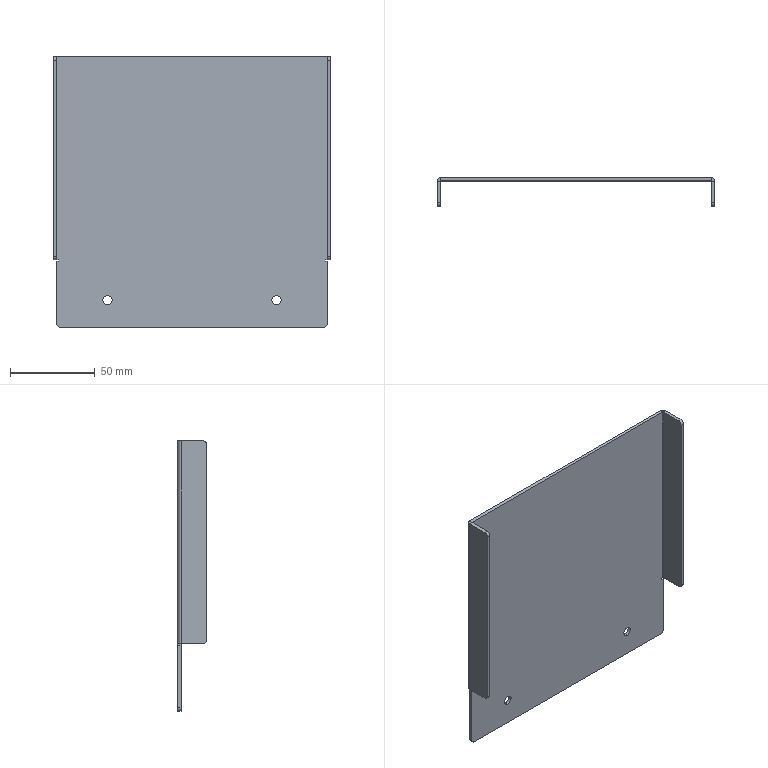Part | STEP file | 1 solid | 40 faces | box 164 x 17 x 160 mm | volume 59024 mm3 | plane 26 | cylinder 14 | commonest cylinder face diameters 4 x6 5.5 x4 0.2 x2 4.2 x2